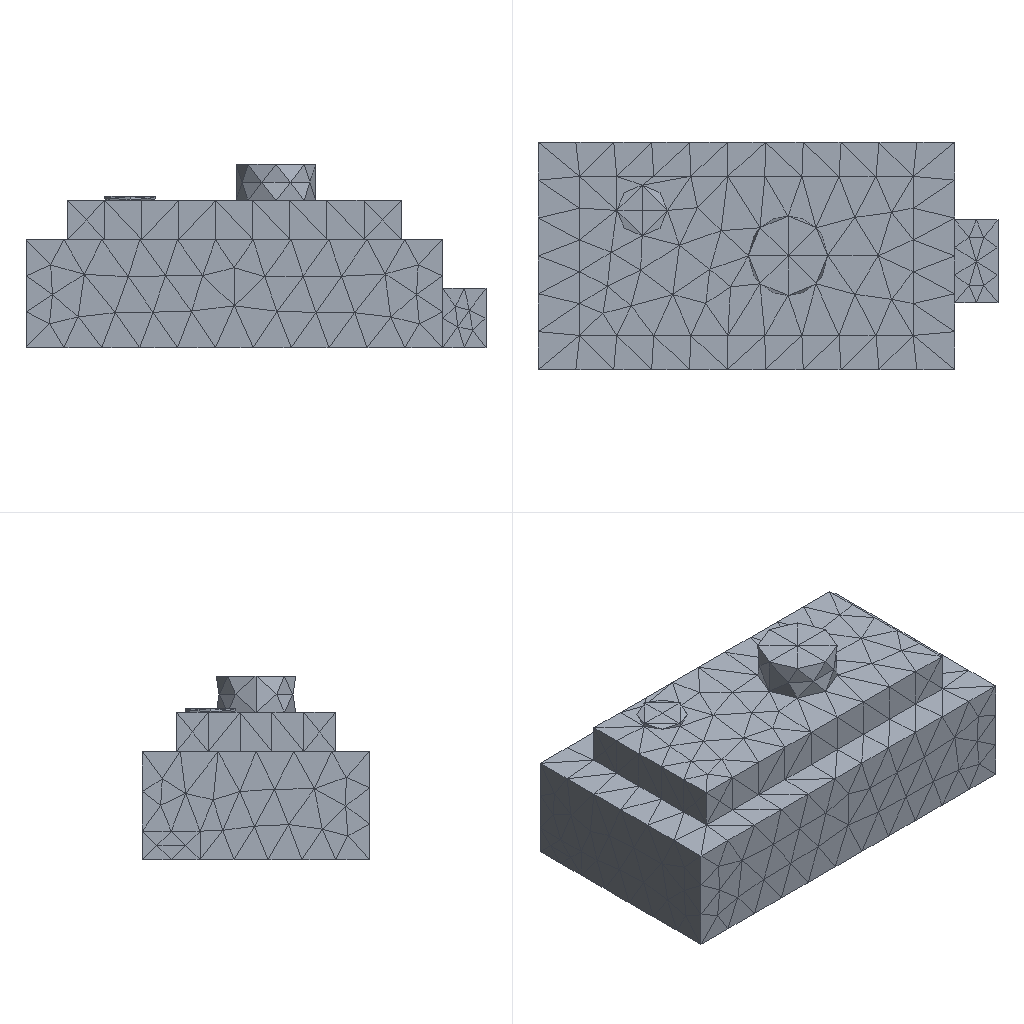Simulation study | ansys mapdl
Set-up summary:
category,name,step,type,value,unit,region
solver,ansys_mapdl
units,mm-N-s-tonne (MPa),,inferred,E=210000 density=
analysis,model,,static
mesh,nodes,,,4040
mesh,elements,,,2386
element_type,SOLID187,,,2386
material,mat 1,,E,210000
material,mat 1,,nu,0.3
load,,model,body load temp,,,all
load,,model,force,"1000 [dir=(0, 0, -1) n=108]",,node list
bc,,model,fixed,"[dofs=UX,UY,UZ n=4602]",,node list
Ansys APDL input file, long lists of numbers shortened:
/COM,ANSYS RELEASE 2026 R1           BUILD 26.1      UP20260202       09:09:39
/PREP7
/NOPR
/TITLE,2
ANTYPE, 0
*IF,_CDRDOFF,EQ,1,THEN     !if solid model was read in
_CDRDOFF=             !reset flag, numoffs already performed
*ELSE              !offset database for the following FE model
NUMOFF,NODE,     4040
NUMOFF,ELEM,     2386
NUMOFF,MAT ,        1
NUMOFF,TYPE,        1
*ENDIF
*SET,_RETURN ,  0.
*SET,_STATUS ,  0.
*SET,_UIQR   ,  108.
*SET,__FLOATPARAMETER__,  4040.
DOF,DELETE
ETBLOCK,        1,        1
(2i9,19a9)
        1      187        0        0        0        0        0        0        0        0        0        0        0        0        0        0        0        0        0        0        0
       -1
NBLOCK,6,SOLID,      4040,      4040
(3i9,6e21.13e3)
        1        0        0-4.1775000000000E+001 3.1500000000000E+001 8.0000000000000E+000
! (4039 more lines like these left out)
N,UNBL,LOC,       -1,
EBLOCK,19,SOLID,      2386,      2386
(19i10)
         1         1         1         1         0         0         0         0        10         0         1      1631      1632      1633      1634      1846      1847      1848      1849
! (4771 more lines like these left out)
        -1
MPTEMP,UNBL, 1, 1,  0.    ,
MPDATA,UNBL, 1,EX  ,       1, 1,  210000.000    ,
MPTEMP,UNBL, 1, 1,  0.    ,
MPDATA,UNBL, 1,NUXY,       1, 1, 0.3    ,
MPTEMP,UNBL, 1, 1,  0.    ,
MPDATA,UNBL, 1,PRXY,       1, 1, 0.3    ,
EXTOPT,ATTR,      0,      0,      0
EXTOPT,ESIZE,  0,  0.
EXTOPT,ACLEAR,      0
TREF,  0.
IRLF,  0
BFUNIF,TEMP,_TINY
ACEL,  0.    ,  0.    ,  0.
OMEGA,  0.    ,  0.    ,  0.
DOMEGA,  0.    ,  0.    ,  0.
CGLOC,  0.    ,  0.    ,  0.
CGOMEGA,  0.    ,  0.    ,  0.
DCGOMG,  0.    ,  0.    ,  0.
KUSE,     0
TIME,  0.
ALPHAD,  0.
BETAD,  0.
DMPRAT,  0.
DMPSTR,  0.
CRPLIM, 0.1    ,   0
CRPLIM,  0.    ,   1
NCNV,     0, 1.000000000E+12,     0,  0.    ,  0.
NEQIT,     0
ERESX,DEFA
DBLOCK,      4602
(i9,a6,2(pg16.9))
        1  UX    0.00000000      0.00000000
! (4601 more lines like these left out)
       -1
FBLOCK,       108
(i9,a6,2(pg16.9))
      736  FZ   -9.25925926      0.00000000
! (107 more lines like these left out)
       -1
/GO
FINISH
Results summary:
result,analysis_type_db,,,static,unstated
result,n_sets,,,1,unstated
result,load_steps[0].set,load_step=1,,1,unstated
result,load_steps[0].substep,load_step=1,,1,unstated
result,load_steps[0].time,load_step=1,,1,unstated
result,load_steps[0].freq,load_step=1,,1,unstated
result,load_steps[0].max_usum,load_step=1,,0.000253,unstated
result,load_steps[0].max_seqv,load_step=1,,2.58,unstated
result,load_steps[0].reaction_sum.FX,load_step=1,,-8.55849e-12,unstated
result,load_steps[0].reaction_sum.FY,load_step=1,,-1.67333e-11,unstated
result,load_steps[0].reaction_sum.FZ,load_step=1,,1000,unstated
result,load_steps[0].reaction_sum.MX,load_step=1,,0,unstated
result,load_steps[0].reaction_sum.MY,load_step=1,,0,unstated
result,load_steps[0].reaction_sum.MZ,load_step=1,,0,unstated
result,convergence,,,results present for all listed sets,unstated